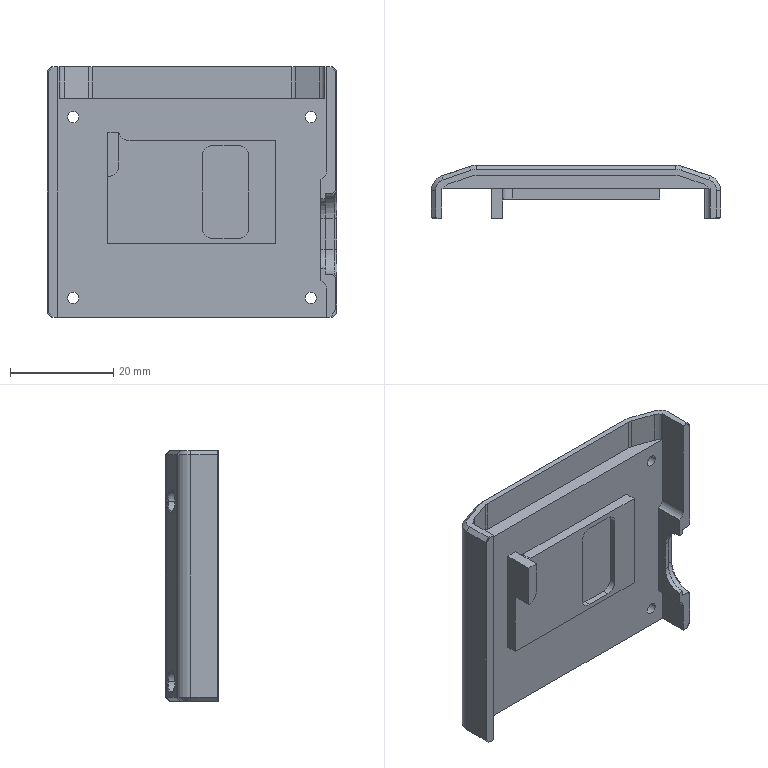Part | SolidWorks | features BaseBody 1 | 1 solid | 158 faces | box 56 x 10.25 x 48.5 mm | volume 11936 mm3 | plane 84 | cylinder 56 | cone 10 | spline 8 | commonest cylinder face diameters 4 x16 2.2 x8 2.5 x8 3 x6 6 x6 8 x6